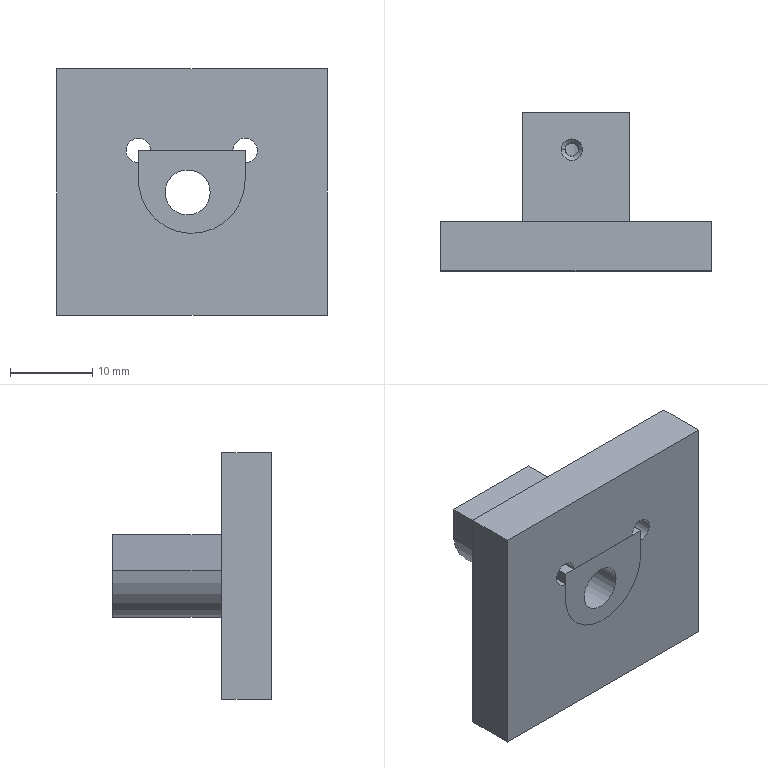NC program | NX | posted with a generic post | part box 32.951 x 19.3 x 30.1 mm
Lines 1 to 40 of 2866:
N10 G17 G21 G94 G90
(FLOOR_WALL_COPY , TOOL : D63)
N12 T01 M6
N14 G54
N16 G17 G0 G90 X-40.953 Y-0.895 B0. C0. S6500 M3
N18 G43 Z30. H1
N20 Z3.
N22 G94 G1 Z0. F1500.
N24 X-37.952 Y-0.834
N26 X37.936 Y0.703
N28 X40.937 Y0.764
N30 Z3.
N32 G0 Z30.
N34 M5
(DRILLING_COPY_1 , TOOL : D6A45)
N36 T07 M6
N38 G54
N40 G17 G0 G90 X-0.5 Y0.05 B0. C0. S5000 M3
N42 G43 Z30. H7
N44 G94 G81 G98 Z-1.3 F250. R3.
N46 G80
N48 G0 X-0.5 Y0.05 Z30.
N50 M5
(DRILLING_COPY_1_COPY , TOOL : 5.5ZT)
N52 T15 M6
N54 G54
N56 G17 G0 G90 X-0.5 Y0.05 B0. C0. S2000 M3
N58 G43 Z30. H15
N60 G94 G83 G98 Z-22.452 F200. Q2. R3.
N62 G80
N64 G0 X-0.5 Y0.05 Z30.
N66 M5